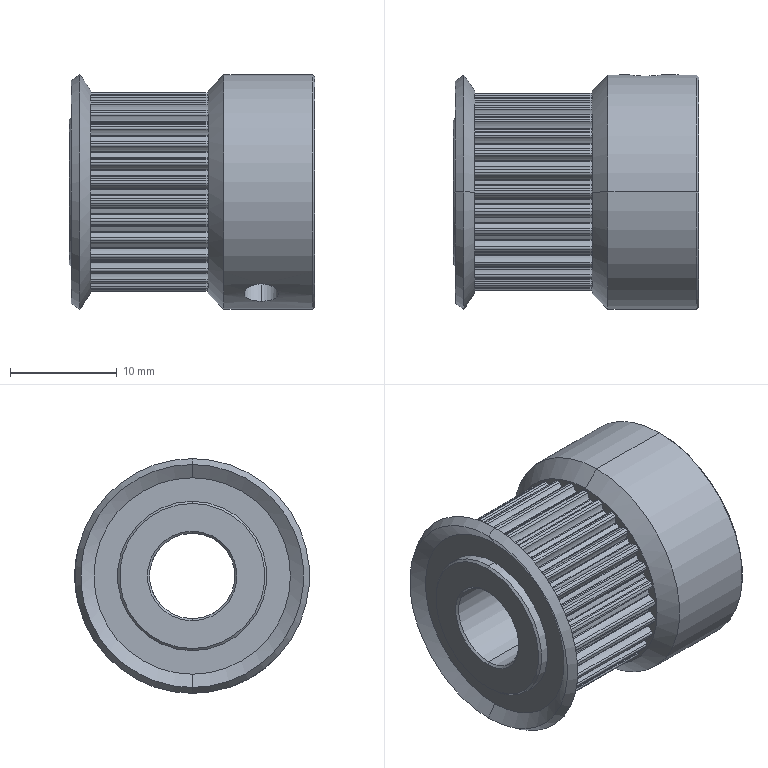Part | SolidWorks | features BaseBody 1 | 1 solid | 296 faces | box 23 x 22 x 22 mm | volume 5708 mm3 | cylinder 275 | cone 16 | plane 5 | commonest cylinder face diameters 0.38 x72 0.2 x68 2.65 x64 18.59 x31 17.07 x30 3.242 x4